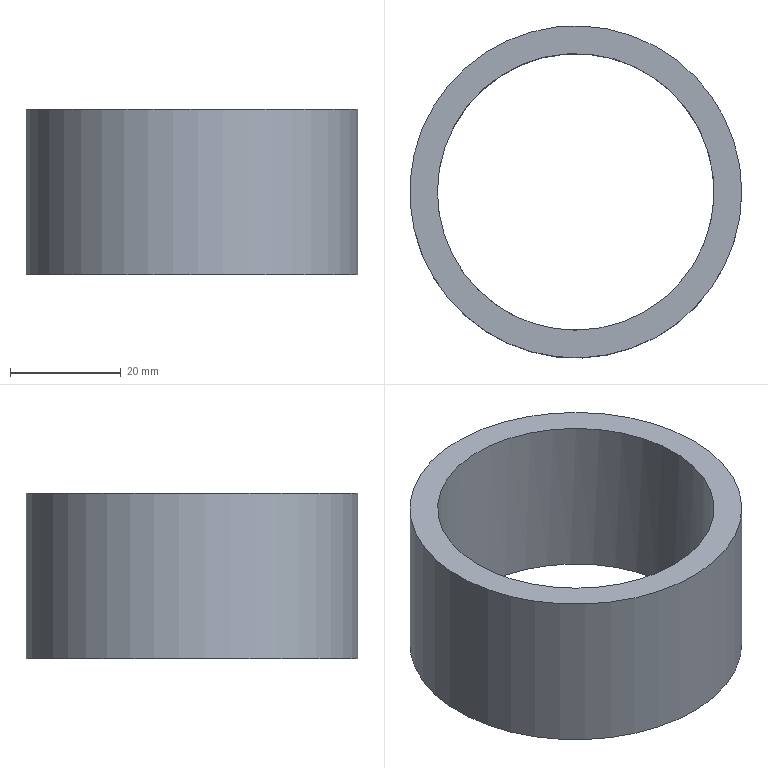Part | STEP file | lll_id518_x_t | 1 solid | 4 faces | box 60 x 60 x 30 mm | volume 25918 mm3 | plane 2 | cylinder 2 | commonest cylinder face diameters 50 x1 60 x1
STEP:
#1=CARTESIAN_POINT('',(3902.435,285.,22.5));
#2=VERTEX_POINT('',#1);
#3=CARTESIAN_POINT('',(3872.435,285.,22.5));
#4=DIRECTION('',(0.,0.,1.));
#5=DIRECTION('',(1.,0.,0.));
#6=AXIS2_PLACEMENT_3D('',#3,#4,#5);
#7=CIRCLE('',#6,30.);
#8=EDGE_CURVE('',#2,#2,#7,.T.);
#9=ORIENTED_EDGE('',*,*,#8,.F.);
#10=EDGE_LOOP('',(#9));
#11=FACE_BOUND('',#10,.T.);
#12=CARTESIAN_POINT('',(3847.435,285.,22.5));
#13=VERTEX_POINT('',#12);
#14=CARTESIAN_POINT('',(3872.435,285.,22.5));
#15=DIRECTION('',(0.,0.,1.));
#16=DIRECTION('',(-1.,0.,0.));
#17=AXIS2_PLACEMENT_3D('',#14,#15,#16);
#18=CIRCLE('',#17,25.);
#19=EDGE_CURVE('',#13,#13,#18,.T.);
#20=ORIENTED_EDGE('',*,*,#19,.T.);
#21=EDGE_LOOP('',(#20));
#22=FACE_BOUND('',#21,.T.);
#23=CARTESIAN_POINT('',(3872.435,285.,22.5));
#24=DIRECTION('',(0.,0.,-1.));
#25=DIRECTION('',(1.,0.,0.));
#26=AXIS2_PLACEMENT_3D('',#23,#24,#25);
#27=PLANE('',#26);
#28=ADVANCED_FACE('',(#11,#22),#27,.T.);
#29=ORIENTED_EDGE('',*,*,#8,.T.);
#30=EDGE_LOOP('',(#29));
#31=FACE_BOUND('',#30,.T.);
#32=CARTESIAN_POINT('',(3902.435,285.,52.5));
#33=VERTEX_POINT('',#32);
#34=CARTESIAN_POINT('',(3872.435,285.,52.5));
#35=DIRECTION('',(0.,0.,1.));
#36=DIRECTION('',(1.,0.,0.));
#37=AXIS2_PLACEMENT_3D('',#34,#35,#36);
#38=CIRCLE('',#37,30.);
#39=EDGE_CURVE('',#33,#33,#38,.T.);
#40=ORIENTED_EDGE('',*,*,#39,.F.);
#41=EDGE_LOOP('',(#40));
#42=FACE_BOUND('',#41,.T.);
#43=CARTESIAN_POINT('',(3872.435,285.,52.5));
#44=DIRECTION('',(0.,0.,-1.));
#45=DIRECTION('',(-1.,0.,0.));
#46=AXIS2_PLACEMENT_3D('',#43,#44,#45);
#47=CYLINDRICAL_SURFACE('',#46,30.);
#48=ADVANCED_FACE('',(#31,#42),#47,.T.);
#49=CARTESIAN_POINT('',(3872.435,260.,52.5));
#50=VERTEX_POINT('',#49);
#51=CARTESIAN_POINT('',(3872.435,285.,52.5));
#52=DIRECTION('',(0.,0.,-1.));
#53=DIRECTION('',(0.,-1.,0.));
#54=AXIS2_PLACEMENT_3D('',#51,#52,#53);
#55=CIRCLE('',#54,25.);
#56=EDGE_CURVE('',#50,#50,#55,.T.);
#57=ORIENTED_EDGE('',*,*,#56,.F.);
#58=EDGE_LOOP('',(#57));
#59=FACE_BOUND('',#58,.T.);
#60=ORIENTED_EDGE('',*,*,#19,.F.);
#61=EDGE_LOOP('',(#60));
#62=FACE_BOUND('',#61,.T.);
#63=CARTESIAN_POINT('',(3872.435,285.,23.5));
#64=DIRECTION('',(0.,0.,-1.));
#65=DIRECTION('',(-1.,0.,0.));
#66=AXIS2_PLACEMENT_3D('',#63,#64,#65);
#67=CYLINDRICAL_SURFACE('',#66,25.);
#68=ADVANCED_FACE('',(#59,#62),#67,.F.);
#69=ORIENTED_EDGE('',*,*,#56,.T.);
#70=EDGE_LOOP('',(#69));
#71=FACE_BOUND('',#70,.T.);
#72=ORIENTED_EDGE('',*,*,#39,.T.);
#73=EDGE_LOOP('',(#72));
#74=FACE_BOUND('',#73,.T.);
#75=CARTESIAN_POINT('',(5722.435,-23.,52.5));
#76=DIRECTION('',(0.,0.,1.));
#77=DIRECTION('',(1.,0.,0.));
#78=AXIS2_PLACEMENT_3D('',#75,#76,#77);
#79=PLANE('',#78);
#80=ADVANCED_FACE('',(#71,#74),#79,.T.);
#81=CLOSED_SHELL('',(#28,#48,#68,#80));
#82=MANIFOLD_SOLID_BREP('',#81);
#83=(LENGTH_UNIT()NAMED_UNIT(*)SI_UNIT(.MILLI.,.METRE.));
#84=UNCERTAINTY_MEASURE_WITH_UNIT(LENGTH_MEASURE(0.00002),#83,'','');
#85=(NAMED_UNIT(*)PLANE_ANGLE_UNIT()SI_UNIT($,.RADIAN.));
#86=PLANE_ANGLE_MEASURE_WITH_UNIT(PLANE_ANGLE_MEASURE(0.01745),#85);
#87=DIMENSIONAL_EXPONENTS(0.,0.,0.,0.,0.,0.,0.);
#88=(CONVERSION_BASED_UNIT('DEGREE',#86)NAMED_UNIT(#87)PLANE_ANGLE_UNIT());
#89=(NAMED_UNIT(*)SI_UNIT($,.STERADIAN.)SOLID_ANGLE_UNIT());
#90=(GEOMETRIC_REPRESENTATION_CONTEXT(3)GLOBAL_UNCERTAINTY_ASSIGNED_CONTEXT((#84))GLOBAL_UNIT_ASSIGNED_CONTEXT((#83,#88,#89))REPRESENTATION_CONTEXT('',''));
#91=ADVANCED_BREP_SHAPE_REPRESENTATION('',(#82),#90);